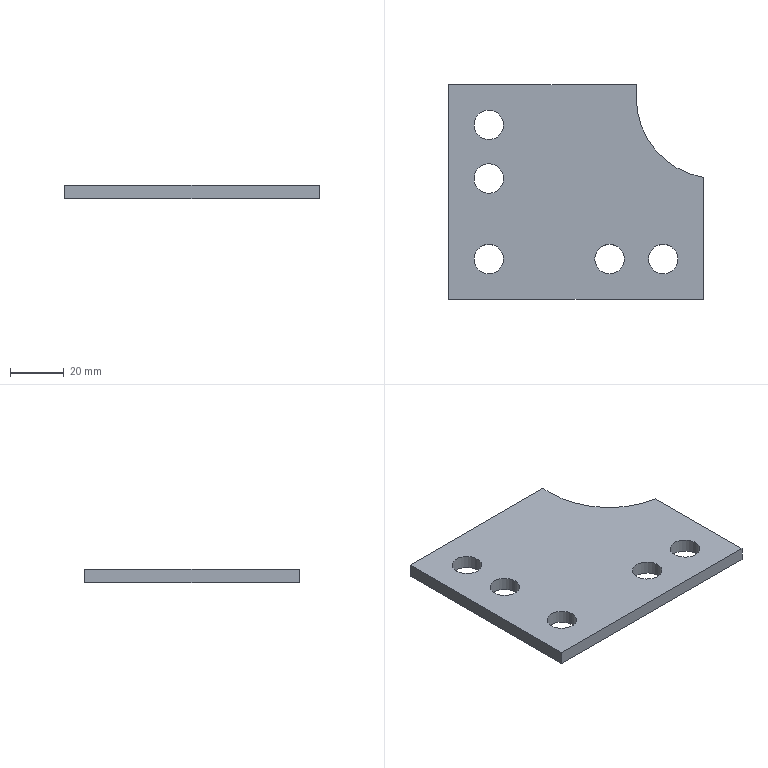Part | NX | features solid 2 | 1 solid | 13 faces | box 95 x 80 x 5 mm | volume 32211 mm3 | plane 7 | cylinder 6 | commonest cylinder face diameters 11 x5 60 x1
STEP:
#1=CARTESIAN_POINT('',(-465.,245.,114.));
#2=VERTEX_POINT('',#1);
#3=CARTESIAN_POINT('',(-395.,245.,114.));
#4=VERTEX_POINT('',#3);
#5=CARTESIAN_POINT('',(-465.,245.,114.));
#6=DIRECTION('',(1.,0.,0.));
#7=VECTOR('',#6,1000.);
#8=LINE('',#5,#7);
#9=EDGE_CURVE('',#2,#4,#8,.T.);
#10=ORIENTED_EDGE('',*,*,#9,.T.);
#11=CARTESIAN_POINT('',(-395.,245.,109.));
#12=VERTEX_POINT('',#11);
#13=CARTESIAN_POINT('',(-395.,245.,114.));
#14=DIRECTION('',(0.,0.,-1.));
#15=VECTOR('',#14,1000.);
#16=LINE('',#13,#15);
#17=EDGE_CURVE('',#4,#12,#16,.T.);
#18=ORIENTED_EDGE('',*,*,#17,.T.);
#19=CARTESIAN_POINT('',(-465.,245.,109.));
#20=VERTEX_POINT('',#19);
#21=CARTESIAN_POINT('',(-465.,245.,109.));
#22=DIRECTION('',(1.,0.,0.));
#23=VECTOR('',#22,1000.);
#24=LINE('',#21,#23);
#25=EDGE_CURVE('',#20,#12,#24,.T.);
#26=ORIENTED_EDGE('',*,*,#25,.F.);
#27=CARTESIAN_POINT('',(-465.,245.,114.));
#28=DIRECTION('',(0.,0.,-1.));
#29=VECTOR('',#28,1000.);
#30=LINE('',#27,#29);
#31=EDGE_CURVE('',#2,#20,#30,.T.);
#32=ORIENTED_EDGE('',*,*,#31,.F.);
#33=EDGE_LOOP('',(#10,#18,#26,#32));
#34=FACE_BOUND('',#33,.T.);
#35=CARTESIAN_POINT('',(-465.,245.,114.));
#36=DIRECTION('',(0.,1.,0.));
#37=DIRECTION('',(0.,0.,1.));
#38=AXIS2_PLACEMENT_3D('',#35,#36,#37);
#39=PLANE('',#38);
#40=ADVANCED_FACE('',(#34),#39,.T.);
#41=CARTESIAN_POINT('',(-370.,165.,109.));
#42=VERTEX_POINT('',#41);
#43=CARTESIAN_POINT('',(-370.,210.42,109.));
#44=VERTEX_POINT('',#43);
#45=CARTESIAN_POINT('',(-370.,165.,109.));
#46=DIRECTION('',(0.,1.,0.));
#47=VECTOR('',#46,1000.);
#48=LINE('',#45,#47);
#49=EDGE_CURVE('',#42,#44,#48,.T.);
#50=ORIENTED_EDGE('',*,*,#49,.T.);
#51=CARTESIAN_POINT('',(-370.,210.42,114.));
#52=VERTEX_POINT('',#51);
#53=CARTESIAN_POINT('',(-370.,210.42,-421.));
#54=DIRECTION('',(0.,0.,1.));
#55=VECTOR('',#54,1000.);
#56=LINE('',#53,#55);
#57=EDGE_CURVE('',#44,#52,#56,.T.);
#58=ORIENTED_EDGE('',*,*,#57,.T.);
#59=CARTESIAN_POINT('',(-370.,165.,114.));
#60=VERTEX_POINT('',#59);
#61=CARTESIAN_POINT('',(-370.,165.,114.));
#62=DIRECTION('',(0.,1.,0.));
#63=VECTOR('',#62,1000.);
#64=LINE('',#61,#63);
#65=EDGE_CURVE('',#60,#52,#64,.T.);
#66=ORIENTED_EDGE('',*,*,#65,.F.);
#67=CARTESIAN_POINT('',(-370.,165.,114.));
#68=DIRECTION('',(0.,0.,-1.));
#69=VECTOR('',#68,1000.);
#70=LINE('',#67,#69);
#71=EDGE_CURVE('',#60,#42,#70,.T.);
#72=ORIENTED_EDGE('',*,*,#71,.T.);
#73=EDGE_LOOP('',(#50,#58,#66,#72));
#74=FACE_BOUND('',#73,.T.);
#75=CARTESIAN_POINT('',(-370.,165.,114.));
#76=DIRECTION('',(-1.,0.,0.));
#77=DIRECTION('',(0.,0.,1.));
#78=AXIS2_PLACEMENT_3D('',#75,#76,#77);
#79=PLANE('',#78);
#80=ADVANCED_FACE('',(#74),#79,.F.);
#81=CARTESIAN_POINT('',(-465.,165.,109.));
#82=VERTEX_POINT('',#81);
#83=CARTESIAN_POINT('',(-465.,165.,109.));
#84=DIRECTION('',(0.,1.,0.));
#85=VECTOR('',#84,1000.);
#86=LINE('',#83,#85);
#87=EDGE_CURVE('',#82,#20,#86,.T.);
#88=ORIENTED_EDGE('',*,*,#87,.F.);
#89=CARTESIAN_POINT('',(-465.,165.,114.));
#90=VERTEX_POINT('',#89);
#91=CARTESIAN_POINT('',(-465.,165.,114.));
#92=DIRECTION('',(0.,0.,-1.));
#93=VECTOR('',#92,1000.);
#94=LINE('',#91,#93);
#95=EDGE_CURVE('',#90,#82,#94,.T.);
#96=ORIENTED_EDGE('',*,*,#95,.F.);
#97=CARTESIAN_POINT('',(-465.,165.,114.));
#98=DIRECTION('',(0.,1.,0.));
#99=VECTOR('',#98,1000.);
#100=LINE('',#97,#99);
#101=EDGE_CURVE('',#90,#2,#100,.T.);
#102=ORIENTED_EDGE('',*,*,#101,.T.);
#103=ORIENTED_EDGE('',*,*,#31,.T.);
#104=EDGE_LOOP('',(#88,#96,#102,#103));
#105=FACE_BOUND('',#104,.T.);
#106=CARTESIAN_POINT('',(-465.,165.,114.));
#107=DIRECTION('',(-1.,0.,0.));
#108=DIRECTION('',(0.,0.,1.));
#109=AXIS2_PLACEMENT_3D('',#106,#107,#108);
#110=PLANE('',#109);
#111=ADVANCED_FACE('',(#105),#110,.T.);
#112=CARTESIAN_POINT('',(-465.,165.,109.));
#113=DIRECTION('',(1.,0.,0.));
#114=VECTOR('',#113,1000.);
#115=LINE('',#112,#114);
#116=EDGE_CURVE('',#82,#42,#115,.T.);
#117=ORIENTED_EDGE('',*,*,#116,.T.);
#118=ORIENTED_EDGE('',*,*,#71,.F.);
#119=CARTESIAN_POINT('',(-465.,165.,114.));
#120=DIRECTION('',(1.,0.,0.));
#121=VECTOR('',#120,1000.);
#122=LINE('',#119,#121);
#123=EDGE_CURVE('',#90,#60,#122,.T.);
#124=ORIENTED_EDGE('',*,*,#123,.F.);
#125=ORIENTED_EDGE('',*,*,#95,.T.);
#126=EDGE_LOOP('',(#117,#118,#124,#125));
#127=FACE_BOUND('',#126,.T.);
#128=CARTESIAN_POINT('',(-465.,165.,114.));
#129=DIRECTION('',(0.,1.,0.));
#130=DIRECTION('',(0.,0.,1.));
#131=AXIS2_PLACEMENT_3D('',#128,#129,#130);
#132=PLANE('',#131);
#133=ADVANCED_FACE('',(#127),#132,.F.);
#134=CARTESIAN_POINT('',(-410.5,180.,114.));
#135=VERTEX_POINT('',#134);
#136=CARTESIAN_POINT('',(-405.,180.,114.));
#137=DIRECTION('',(0.,0.,-1.));
#138=DIRECTION('',(-1.,0.,0.));
#139=AXIS2_PLACEMENT_3D('',#136,#137,#138);
#140=CIRCLE('',#139,5.5);
#141=EDGE_CURVE('',#135,#135,#140,.T.);
#142=ORIENTED_EDGE('',*,*,#141,.T.);
#143=EDGE_LOOP('',(#142));
#144=FACE_BOUND('',#143,.T.);
#145=CARTESIAN_POINT('',(-455.5,210.,114.));
#146=VERTEX_POINT('',#145);
#147=CARTESIAN_POINT('',(-450.,210.,114.));
#148=DIRECTION('',(0.,0.,-1.));
#149=DIRECTION('',(-1.,0.,0.));
#150=AXIS2_PLACEMENT_3D('',#147,#148,#149);
#151=CIRCLE('',#150,5.5);
#152=EDGE_CURVE('',#146,#146,#151,.T.);
#153=ORIENTED_EDGE('',*,*,#152,.T.);
#154=EDGE_LOOP('',(#153));
#155=FACE_BOUND('',#154,.T.);
#156=CARTESIAN_POINT('',(-390.5,180.,114.));
#157=VERTEX_POINT('',#156);
#158=CARTESIAN_POINT('',(-385.,180.,114.));
#159=DIRECTION('',(0.,0.,-1.));
#160=DIRECTION('',(-1.,0.,0.));
#161=AXIS2_PLACEMENT_3D('',#158,#159,#160);
#162=CIRCLE('',#161,5.5);
#163=EDGE_CURVE('',#157,#157,#162,.T.);
#164=ORIENTED_EDGE('',*,*,#163,.T.);
#165=EDGE_LOOP('',(#164));
#166=FACE_BOUND('',#165,.T.);
#167=CARTESIAN_POINT('',(-455.5,180.,114.));
#168=VERTEX_POINT('',#167);
#169=CARTESIAN_POINT('',(-450.,180.,114.));
#170=DIRECTION('',(0.,0.,-1.));
#171=DIRECTION('',(-1.,0.,0.));
#172=AXIS2_PLACEMENT_3D('',#169,#170,#171);
#173=CIRCLE('',#172,5.5);
#174=EDGE_CURVE('',#168,#168,#173,.T.);
#175=ORIENTED_EDGE('',*,*,#174,.T.);
#176=EDGE_LOOP('',(#175));
#177=FACE_BOUND('',#176,.T.);
#178=CARTESIAN_POINT('',(-455.5,230.,114.));
#179=VERTEX_POINT('',#178);
#180=CARTESIAN_POINT('',(-450.,230.,114.));
#181=DIRECTION('',(0.,0.,-1.));
#182=DIRECTION('',(-1.,0.,0.));
#183=AXIS2_PLACEMENT_3D('',#180,#181,#182);
#184=CIRCLE('',#183,5.5);
#185=EDGE_CURVE('',#179,#179,#184,.T.);
#186=ORIENTED_EDGE('',*,*,#185,.T.);
#187=EDGE_LOOP('',(#186));
#188=FACE_BOUND('',#187,.T.);
#189=ORIENTED_EDGE('',*,*,#65,.T.);
#190=CARTESIAN_POINT('',(-395.,240.,114.));
#191=VERTEX_POINT('',#190);
#192=CARTESIAN_POINT('',(-365.,240.,114.));
#193=DIRECTION('',(0.,0.,-1.));
#194=DIRECTION('',(-1.,0.,0.));
#195=AXIS2_PLACEMENT_3D('',#192,#193,#194);
#196=CIRCLE('',#195,30.);
#197=EDGE_CURVE('',#52,#191,#196,.T.);
#198=ORIENTED_EDGE('',*,*,#197,.T.);
#199=CARTESIAN_POINT('',(-395.,245.,114.));
#200=DIRECTION('',(0.,-1.,0.));
#201=VECTOR('',#200,1000.);
#202=LINE('',#199,#201);
#203=EDGE_CURVE('',#4,#191,#202,.T.);
#204=ORIENTED_EDGE('',*,*,#203,.F.);
#205=ORIENTED_EDGE('',*,*,#9,.F.);
#206=ORIENTED_EDGE('',*,*,#101,.F.);
#207=ORIENTED_EDGE('',*,*,#123,.T.);
#208=EDGE_LOOP('',(#189,#198,#204,#205,#206,#207));
#209=FACE_BOUND('',#208,.T.);
#210=CARTESIAN_POINT('',(-370.,245.,114.));
#211=DIRECTION('',(0.,0.,-1.));
#212=DIRECTION('',(-1.,0.,0.));
#213=AXIS2_PLACEMENT_3D('',#210,#211,#212);
#214=PLANE('',#213);
#215=ADVANCED_FACE('',(#144,#155,#166,#177,#188,#209),#214,.F.);
#216=CARTESIAN_POINT('',(-395.,240.,109.));
#217=VERTEX_POINT('',#216);
#218=CARTESIAN_POINT('',(-365.,240.,109.));
#219=DIRECTION('',(0.,0.,-1.));
#220=DIRECTION('',(-1.,0.,0.));
#221=AXIS2_PLACEMENT_3D('',#218,#219,#220);
#222=CIRCLE('',#221,30.);
#223=EDGE_CURVE('',#44,#217,#222,.T.);
#224=ORIENTED_EDGE('',*,*,#223,.F.);
#225=ORIENTED_EDGE('',*,*,#49,.F.);
#226=ORIENTED_EDGE('',*,*,#116,.F.);
#227=ORIENTED_EDGE('',*,*,#87,.T.);
#228=ORIENTED_EDGE('',*,*,#25,.T.);
#229=CARTESIAN_POINT('',(-395.,245.,109.));
#230=DIRECTION('',(0.,-1.,0.));
#231=VECTOR('',#230,1000.);
#232=LINE('',#229,#231);
#233=EDGE_CURVE('',#12,#217,#232,.T.);
#234=ORIENTED_EDGE('',*,*,#233,.T.);
#235=EDGE_LOOP('',(#224,#225,#226,#227,#228,#234));
#236=FACE_BOUND('',#235,.T.);
#237=CARTESIAN_POINT('',(-410.5,180.,109.));
#238=VERTEX_POINT('',#237);
#239=CARTESIAN_POINT('',(-405.,180.,109.));
#240=DIRECTION('',(0.,0.,-1.));
#241=DIRECTION('',(-1.,0.,0.));
#242=AXIS2_PLACEMENT_3D('',#239,#240,#241);
#243=CIRCLE('',#242,5.5);
#244=EDGE_CURVE('',#238,#238,#243,.T.);
#245=ORIENTED_EDGE('',*,*,#244,.F.);
#246=EDGE_LOOP('',(#245));
#247=FACE_BOUND('',#246,.T.);
#248=CARTESIAN_POINT('',(-455.5,210.,109.));
#249=VERTEX_POINT('',#248);
#250=CARTESIAN_POINT('',(-450.,210.,109.));
#251=DIRECTION('',(0.,0.,-1.));
#252=DIRECTION('',(-1.,0.,0.));
#253=AXIS2_PLACEMENT_3D('',#250,#251,#252);
#254=CIRCLE('',#253,5.5);
#255=EDGE_CURVE('',#249,#249,#254,.T.);
#256=ORIENTED_EDGE('',*,*,#255,.F.);
#257=EDGE_LOOP('',(#256));
#258=FACE_BOUND('',#257,.T.);
#259=CARTESIAN_POINT('',(-390.5,180.,109.));
#260=VERTEX_POINT('',#259);
#261=CARTESIAN_POINT('',(-385.,180.,109.));
#262=DIRECTION('',(0.,0.,-1.));
#263=DIRECTION('',(-1.,0.,0.));
#264=AXIS2_PLACEMENT_3D('',#261,#262,#263);
#265=CIRCLE('',#264,5.5);
#266=EDGE_CURVE('',#260,#260,#265,.T.);
#267=ORIENTED_EDGE('',*,*,#266,.F.);
#268=EDGE_LOOP('',(#267));
#269=FACE_BOUND('',#268,.T.);
#270=CARTESIAN_POINT('',(-455.5,180.,109.));
#271=VERTEX_POINT('',#270);
#272=CARTESIAN_POINT('',(-450.,180.,109.));
#273=DIRECTION('',(0.,0.,-1.));
#274=DIRECTION('',(-1.,0.,0.));
#275=AXIS2_PLACEMENT_3D('',#272,#273,#274);
#276=CIRCLE('',#275,5.5);
#277=EDGE_CURVE('',#271,#271,#276,.T.);
#278=ORIENTED_EDGE('',*,*,#277,.F.);
#279=EDGE_LOOP('',(#278));
#280=FACE_BOUND('',#279,.T.);
#281=CARTESIAN_POINT('',(-455.5,230.,109.));
#282=VERTEX_POINT('',#281);
#283=CARTESIAN_POINT('',(-450.,230.,109.));
#284=DIRECTION('',(0.,0.,-1.));
#285=DIRECTION('',(-1.,0.,0.));
#286=AXIS2_PLACEMENT_3D('',#283,#284,#285);
#287=CIRCLE('',#286,5.5);
#288=EDGE_CURVE('',#282,#282,#287,.T.);
#289=ORIENTED_EDGE('',*,*,#288,.F.);
#290=EDGE_LOOP('',(#289));
#291=FACE_BOUND('',#290,.T.);
#292=CARTESIAN_POINT('',(-370.,245.,109.));
#293=DIRECTION('',(0.,0.,-1.));
#294=DIRECTION('',(-1.,0.,0.));
#295=AXIS2_PLACEMENT_3D('',#292,#293,#294);
#296=PLANE('',#295);
#297=ADVANCED_FACE('',(#236,#247,#258,#269,#280,#291),#296,.T.);
#298=ORIENTED_EDGE('',*,*,#288,.T.);
#299=EDGE_LOOP('',(#298));
#300=FACE_BOUND('',#299,.T.);
#301=ORIENTED_EDGE('',*,*,#185,.F.);
#302=EDGE_LOOP('',(#301));
#303=FACE_BOUND('',#302,.T.);
#304=CARTESIAN_POINT('',(-450.,230.,-111.));
#305=DIRECTION('',(0.,0.,1.));
#306=DIRECTION('',(1.,0.,0.));
#307=AXIS2_PLACEMENT_3D('',#304,#305,#306);
#308=CYLINDRICAL_SURFACE('',#307,5.5);
#309=ADVANCED_FACE('',(#300,#303),#308,.F.);
#310=ORIENTED_EDGE('',*,*,#277,.T.);
#311=EDGE_LOOP('',(#310));
#312=FACE_BOUND('',#311,.T.);
#313=ORIENTED_EDGE('',*,*,#174,.F.);
#314=EDGE_LOOP('',(#313));
#315=FACE_BOUND('',#314,.T.);
#316=CARTESIAN_POINT('',(-450.,180.,-111.));
#317=DIRECTION('',(0.,0.,1.));
#318=DIRECTION('',(1.,0.,0.));
#319=AXIS2_PLACEMENT_3D('',#316,#317,#318);
#320=CYLINDRICAL_SURFACE('',#319,5.5);
#321=ADVANCED_FACE('',(#312,#315),#320,.F.);
#322=ORIENTED_EDGE('',*,*,#266,.T.);
#323=EDGE_LOOP('',(#322));
#324=FACE_BOUND('',#323,.T.);
#325=ORIENTED_EDGE('',*,*,#163,.F.);
#326=EDGE_LOOP('',(#325));
#327=FACE_BOUND('',#326,.T.);
#328=CARTESIAN_POINT('',(-385.,180.,-111.));
#329=DIRECTION('',(0.,0.,1.));
#330=DIRECTION('',(1.,0.,0.));
#331=AXIS2_PLACEMENT_3D('',#328,#329,#330);
#332=CYLINDRICAL_SURFACE('',#331,5.5);
#333=ADVANCED_FACE('',(#324,#327),#332,.F.);
#334=ORIENTED_EDGE('',*,*,#255,.T.);
#335=EDGE_LOOP('',(#334));
#336=FACE_BOUND('',#335,.T.);
#337=ORIENTED_EDGE('',*,*,#152,.F.);
#338=EDGE_LOOP('',(#337));
#339=FACE_BOUND('',#338,.T.);
#340=CARTESIAN_POINT('',(-450.,210.,-111.));
#341=DIRECTION('',(0.,0.,1.));
#342=DIRECTION('',(1.,0.,0.));
#343=AXIS2_PLACEMENT_3D('',#340,#341,#342);
#344=CYLINDRICAL_SURFACE('',#343,5.5);
#345=ADVANCED_FACE('',(#336,#339),#344,.F.);
#346=ORIENTED_EDGE('',*,*,#244,.T.);
#347=EDGE_LOOP('',(#346));
#348=FACE_BOUND('',#347,.T.);
#349=ORIENTED_EDGE('',*,*,#141,.F.);
#350=EDGE_LOOP('',(#349));
#351=FACE_BOUND('',#350,.T.);
#352=CARTESIAN_POINT('',(-405.,180.,-111.));
#353=DIRECTION('',(0.,0.,1.));
#354=DIRECTION('',(1.,0.,0.));
#355=AXIS2_PLACEMENT_3D('',#352,#353,#354);
#356=CYLINDRICAL_SURFACE('',#355,5.5);
#357=ADVANCED_FACE('',(#348,#351),#356,.F.);
#358=ORIENTED_EDGE('',*,*,#57,.F.);
#359=ORIENTED_EDGE('',*,*,#223,.T.);
#360=CARTESIAN_POINT('',(-395.,240.,-421.));
#361=DIRECTION('',(0.,0.,1.));
#362=VECTOR('',#361,1000.);
#363=LINE('',#360,#362);
#364=EDGE_CURVE('',#217,#191,#363,.T.);
#365=ORIENTED_EDGE('',*,*,#364,.T.);
#366=ORIENTED_EDGE('',*,*,#197,.F.);
#367=EDGE_LOOP('',(#358,#359,#365,#366));
#368=FACE_BOUND('',#367,.T.);
#369=CARTESIAN_POINT('',(-365.,240.,-421.));
#370=DIRECTION('',(0.,0.,1.));
#371=DIRECTION('',(1.,0.,0.));
#372=AXIS2_PLACEMENT_3D('',#369,#370,#371);
#373=CYLINDRICAL_SURFACE('',#372,30.);
#374=ADVANCED_FACE('',(#368),#373,.F.);
#375=ORIENTED_EDGE('',*,*,#203,.T.);
#376=ORIENTED_EDGE('',*,*,#364,.F.);
#377=ORIENTED_EDGE('',*,*,#233,.F.);
#378=ORIENTED_EDGE('',*,*,#17,.F.);
#379=EDGE_LOOP('',(#375,#376,#377,#378));
#380=FACE_BOUND('',#379,.T.);
#381=CARTESIAN_POINT('',(-395.,240.,-421.));
#382=DIRECTION('',(1.,0.,0.));
#383=DIRECTION('',(0.,0.,-1.));
#384=AXIS2_PLACEMENT_3D('',#381,#382,#383);
#385=PLANE('',#384);
#386=ADVANCED_FACE('',(#380),#385,.T.);
#387=CLOSED_SHELL('',(#40,#80,#111,#133,#215,#297,#309,#321,#333,#345,#357,#374,#386));
#388=MANIFOLD_SOLID_BREP('',#387);
#389=(LENGTH_UNIT()NAMED_UNIT(*)SI_UNIT(.MILLI.,.METRE.));
#390=UNCERTAINTY_MEASURE_WITH_UNIT(LENGTH_MEASURE(0.00001),#389,'','');
#391=(NAMED_UNIT(*)PLANE_ANGLE_UNIT()SI_UNIT($,.RADIAN.));
#392=(NAMED_UNIT(*)SI_UNIT($,.STERADIAN.)SOLID_ANGLE_UNIT());
#393=(GEOMETRIC_REPRESENTATION_CONTEXT(3)GLOBAL_UNCERTAINTY_ASSIGNED_CONTEXT((#390))GLOBAL_UNIT_ASSIGNED_CONTEXT((#389,#391,#392))REPRESENTATION_CONTEXT('',''));
#394=ADVANCED_BREP_SHAPE_REPRESENTATION('',(#388),#393);